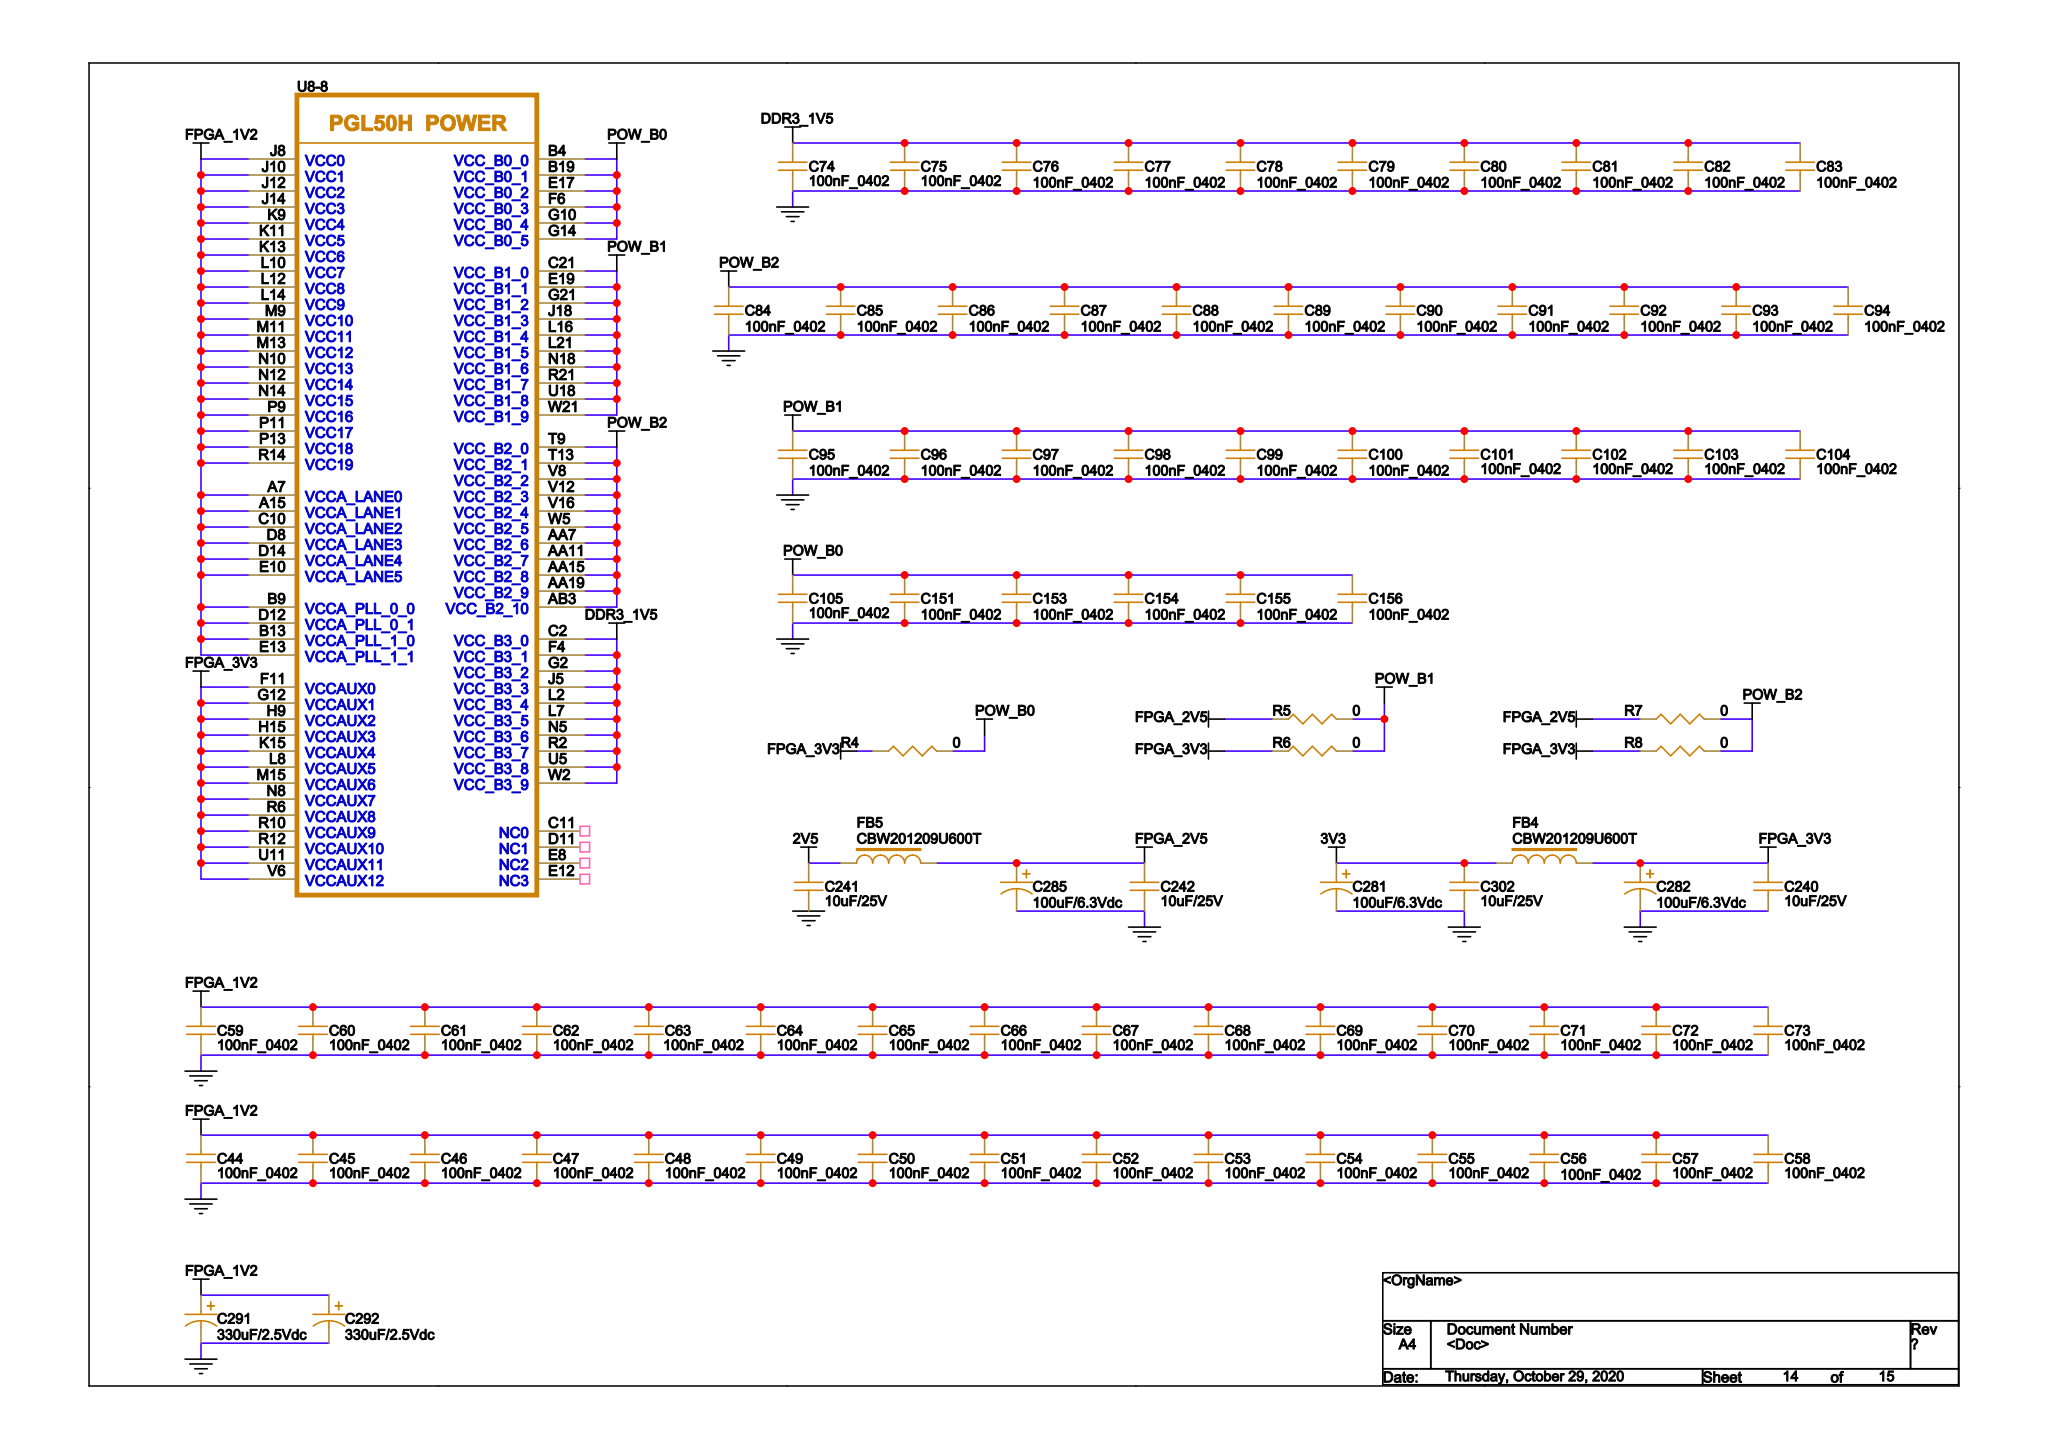Circuit board | Cadence Allegro | 406 parts | 392 nets | one sheet of the schematic
Parts on this sheet (reference | value | footprint):
C44 | 100nF_0402 | C_0402_104
C45 | 100nF_0402 | C_0402_104
C46 | 100nF_0402 | C_0402_104
C47 | 100nF_0402 | C_0402_104
C48 | 100nF_0402 | C_0402_104
C49 | 100nF_0402 | C_0402_104
C50 | 100nF_0402 | C_0402_104
C51 | 100nF_0402 | C_0402_104
C52 | 100nF_0402 | C_0402_104
C53 | 100nF_0402 | C_0402_104
C54 | 100nF_0402 | C_0402_104
C55 | 100nF_0402 | C_0402_104
C56 | 100nF_0402 | C_0402_104
C57 | 100nF_0402 | C_0402_104
C58 | 100nF_0402 | C_0402_104
C59 | 100nF_0402 | C_0402_104
C60 | 100nF_0402 | C_0402_104
C61 | 100nF_0402 | C_0402_104
C62 | 100nF_0402 | C_0402_104
C63 | 100nF_0402 | C_0402_104
C64 | 100nF_0402 | C_0402_104
C65 | 100nF_0402 | C_0402_104
C66 | 100nF_0402 | C_0402_104
C67 | 100nF_0402 | C_0402_104
C68 | 100nF_0402 | C_0402_104
C69 | 100nF_0402 | C_0402_104
C70 | 100nF_0402 | C_0402_104
C71 | 100nF_0402 | C_0402_104
C72 | 100nF_0402 | C_0402_104
C73 | 100nF_0402 | C_0402_104
C74 | 100nF_0402 | C_0402_104
C75 | 100nF_0402 | C_0402_104
C76 | 100nF_0402 | C_0402_104
C77 | 100nF_0402 | C_0402_104
C78 | 100nF_0402 | C_0402_104
C79 | 100nF_0402 | C_0402_104
C80 | 100nF_0402 | C_0402_104
C81 | 100nF_0402 | C_0402_104
C82 | 100nF_0402 | C_0402_104
C83 | 100nF_0402 | C_0402_104
C84 | 100nF_0402 | C_0402_104
C85 | 100nF_0402 | C_0402_104
C86 | 100nF_0402 | C_0402_104
C87 | 100nF_0402 | C_0402_104
C88 | 100nF_0402 | C_0402_104
C89 | 100nF_0402 | C_0402_104
C90 | 100nF_0402 | C_0402_104
C91 | 100nF_0402 | C_0402_104
C92 | 100nF_0402 | C_0402_104
C93 | 100nF_0402 | C_0402_104
C94 | 100nF_0402 | C_0402_104
C95 | 100nF_0402 | C_0402_104
C96 | 100nF_0402 | C_0402_104
C97 | 100nF_0402 | C_0402_104
C98 | 100nF_0402 | C_0402_104
C99 | 100nF_0402 | C_0402_104
C100 | 100nF_0402 | C_0402_104
C101 | 100nF_0402 | C_0402_104
C102 | 100nF_0402 | C_0402_104
C103 | 100nF_0402 | C_0402_104
C104 | 100nF_0402 | C_0402_104
C105 | 100nF_0402 | C_0402_104
C151 | 100nF_0402 | C_0402_104
C153 | 100nF_0402 | C_0402_104
C154 | 100nF_0402 | C_0402_104
C155 | 100nF_0402 | C_0402_104
C156 | 100nF_0402 | C_0402_104
C240 | 10uF/25V | C_0805_106
C241 | 10uF/25V | C_0805_106
C242 | 10uF/25V | C_0805_106
C281 | 100uF/6.3Vdc | C_7343
C282 | 100uF/6.3Vdc | C_7343
C285 | 100uF/6.3Vdc | C_7343
C291 | 330uF/2.5Vdc | C_7343
C292 | 330uF/2.5Vdc | C_7343
C302 | 10uF/25V | C_0805_106
FB4 | CBW201209U600T | L_0805
FB5 | CBW201209U600T | L_0805
J10 | COM_E connector 220X8 FEMALE | JP_220X8PF
R4 | 0 | R_0603
R5 | 0 | R_0603
R6 | 0 | R_0603
R7 | 0 | R_0603
R8 | 0 | R_0603
Nets of these parts (net: part-pin ...):
GND: C44-2 C45-2 C46-2 C47-2 C48-2 C49-2 C50-2 C51-2 C52-2 C53-2 C54-2 C55-2 C56-2 C57-2 C58-2 C59-2 C60-2 C61-2 C62-2 C63-2 C64-2 C65-2 C66-2 C67-2 C68-2 C69-2 C70-2 C71-2 C72-2 C73-2 C74-2 C75-2 C76-2 C77-2 C78-2 C79-2 C80-2 C81-2 C82-2 C83-2 C84-2 C85-2 C86-2 C87-2 C88-2 C89-2 C90-2 C91-2 C92-2 C93-2 C94-2 C95-2 C96-2 C97-2 C98-2 C99-2 C100-2 C101-2 C102-2 C103-2 C104-2 C105-2 C151-2 C153-2 C154-2 C155-2 C156-2 C240-2 C241-2 C242-2 C281-2 C282-2 C285-2 C291-2 C292-2 C302-2 J10-A4 J10-A7 J10-A15 J10-B4
POW_B1: C95-1 C96-1 C97-1 C98-1 C99-1 C100-1 C101-1 C102-1 C103-1 C104-1 R5-2 R6-2
POW_B0: C105-1 C151-1 C153-1 C154-1 C155-1 C156-1 R4-2
FPGA_3V3: C240-1 C282-1 FB4-2 R4-1 R6-1 R8-1
FPGA_1V2: C44-1 C45-1 C46-1 C47-1 C48-1 C49-1 C50-1 C51-1 C52-1 C53-1 C54-1 C55-1 C56-1 C57-1 C58-1 C59-1 C60-1 C61-1 C62-1 C63-1 C64-1 C65-1 C66-1 C67-1 C68-1 C69-1 C70-1 C71-1 C72-1 C73-1 C291-1 C292-1
DDR3_1V5: C74-1 C75-1 C76-1 C77-1 C78-1 C79-1 C80-1 C81-1 C82-1 C83-1
POW_B2: C84-1 C85-1 C86-1 C87-1 C88-1 C89-1 C90-1 C91-1 C92-1 C93-1 C94-1 R7-2 R8-2
3V3: C281-1 C302-1 FB4-1
2V5: C241-1 FB5-1
FPGA_2V5: C242-1 C285-1 FB5-2 R5-1 R7-1